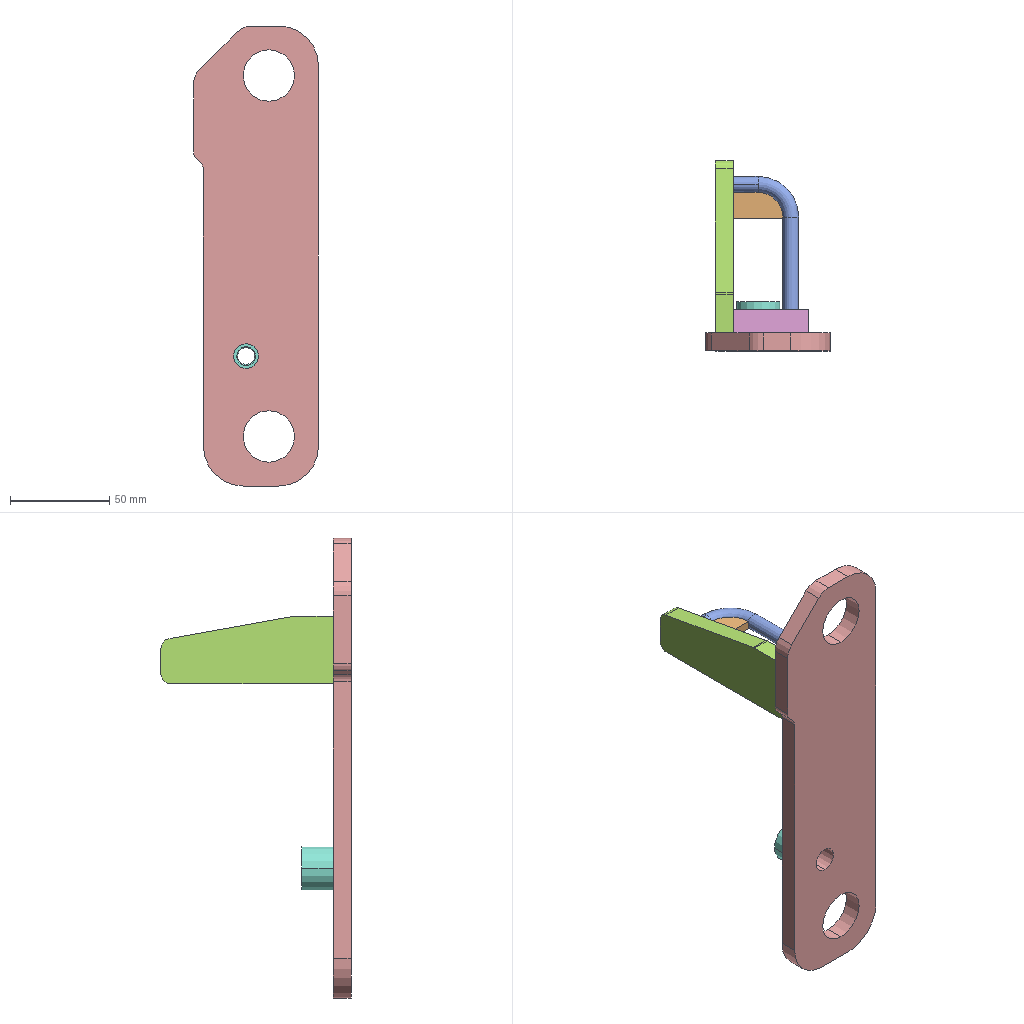Assembly | SolidWorks | 6 different items | 6 placed | box 63 x 96 x 232 mm
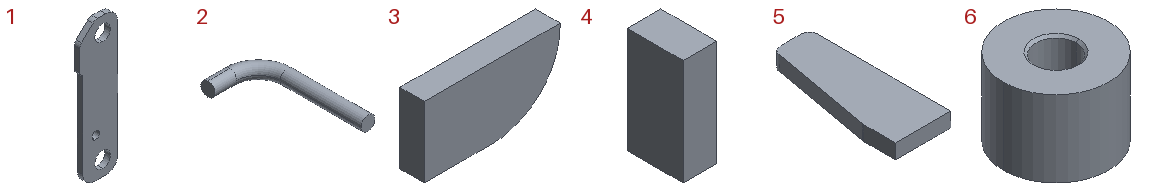Parts list (item | quantity | size | volume | features):
1 | x1 | 63 x 9 x 232 mm | 108334 mm3 | features Extrusion 1
2 | x1 | 33 x 67 x 8 mm | 4268 mm3 | features Sweep 1
3 | x1 | 25 x 4.5 x 13 mm | 1312 mm3 | features Extrusion 1
4 | x1 | 12 x 20 x 38 mm | 9120 mm3 | features Extrusion 1
5 | x1 | 34 x 87 x 9 mm | 22924 mm3 | features Extrusion 1
6 | x1 | 22 x 22 x 16 mm | 5167 mm3 | features Chamfer 1, Extrusion 1, ICE 1
Mates (type | each side: item.copy, entity, surface, feature):
Coincident | 1.1 face plane Boss-Extrude1 | 5.1 face plane Boss-Extrude1
DistanceDim | 1.1 face plane Boss-Extrude1 | 5.1 face plane Boss-Extrude1
Coincident | 2.1 face plane Sweep1 | 5.1 face plane Boss-Extrude1
Coincident | 1.1 face plane Boss-Extrude1 | 4.1 face plane Boss-Extrude1
DistanceDim | 4.1 face plane Boss-Extrude1 | 1.1 face plane Boss-Extrude1
Coincident | 5.1 face plane Boss-Extrude1 | 4.1 face plane Boss-Extrude1
Coincident | 2.1 face plane Sweep1 | 4.1 face plane Boss-Extrude1
Coincident | 1.1 face plane Boss-Extrude1 | 6.1 face plane Boss-Extrude1
Concentric | 1.1 face cylinder Boss-Extrude1 | 6.1 face cylinder Cut-Extrude1
Coincident | 5.1 face plane Boss-Extrude1 | 3.1 face plane Boss-Extrude1
Coincident | 2.1 plane | 3.1 plane
Tangent | 2.1 face cylinder Sweep1 | 3.1 face plane Boss-Extrude1